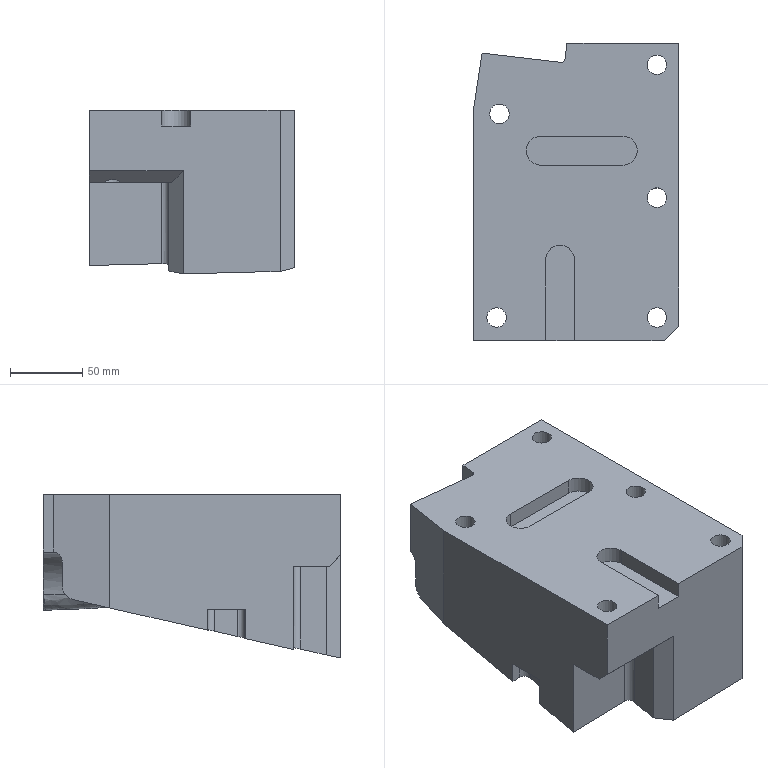Part | NX | features 8 2 | 1 solid | 90 faces | box 142 x 206 x 113.403 mm | volume 2286065 mm3 | plane 37 | cylinder 30 | spline 19 | torus 2 | cone 2 | commonest cylinder face diameters 20 x8 10 x7 13.5 x5 14 x3 8.5 x2 6 x1